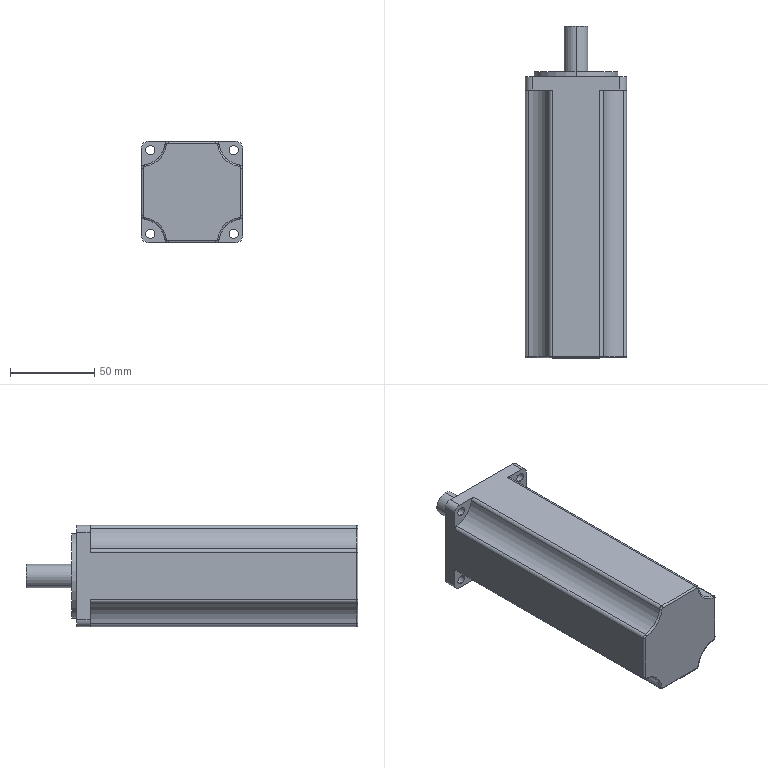Part | SolidWorks | features BaseBody 1 | 1 solid | 56 faces | box 60 x 196.8 x 60 mm | volume 510939 mm3 | cylinder 32 | plane 12 | torus 12 | commonest cylinder face diameters 4 x8 5.5 x8 2 x4 8 x4 28 x4 14 x2